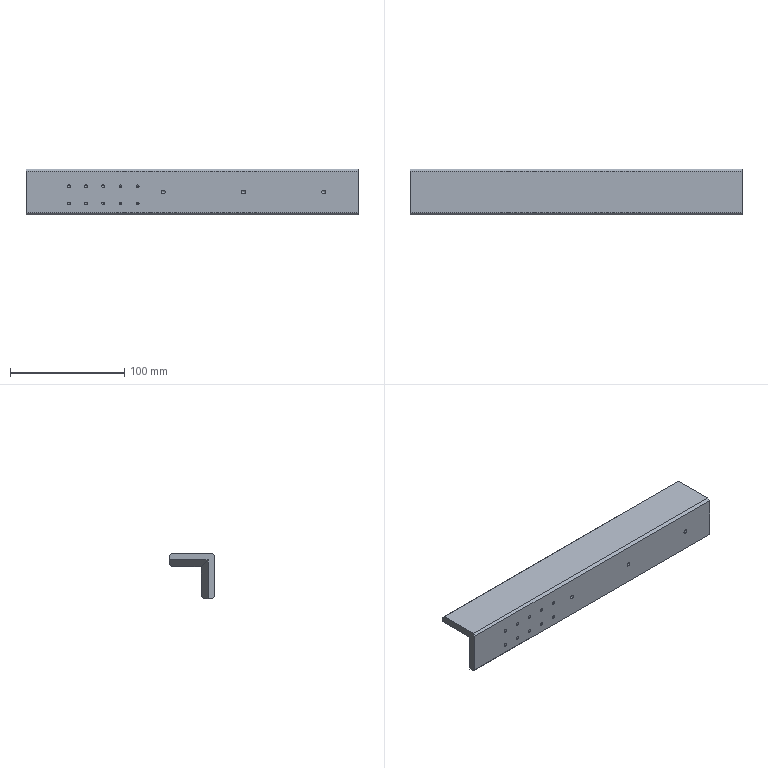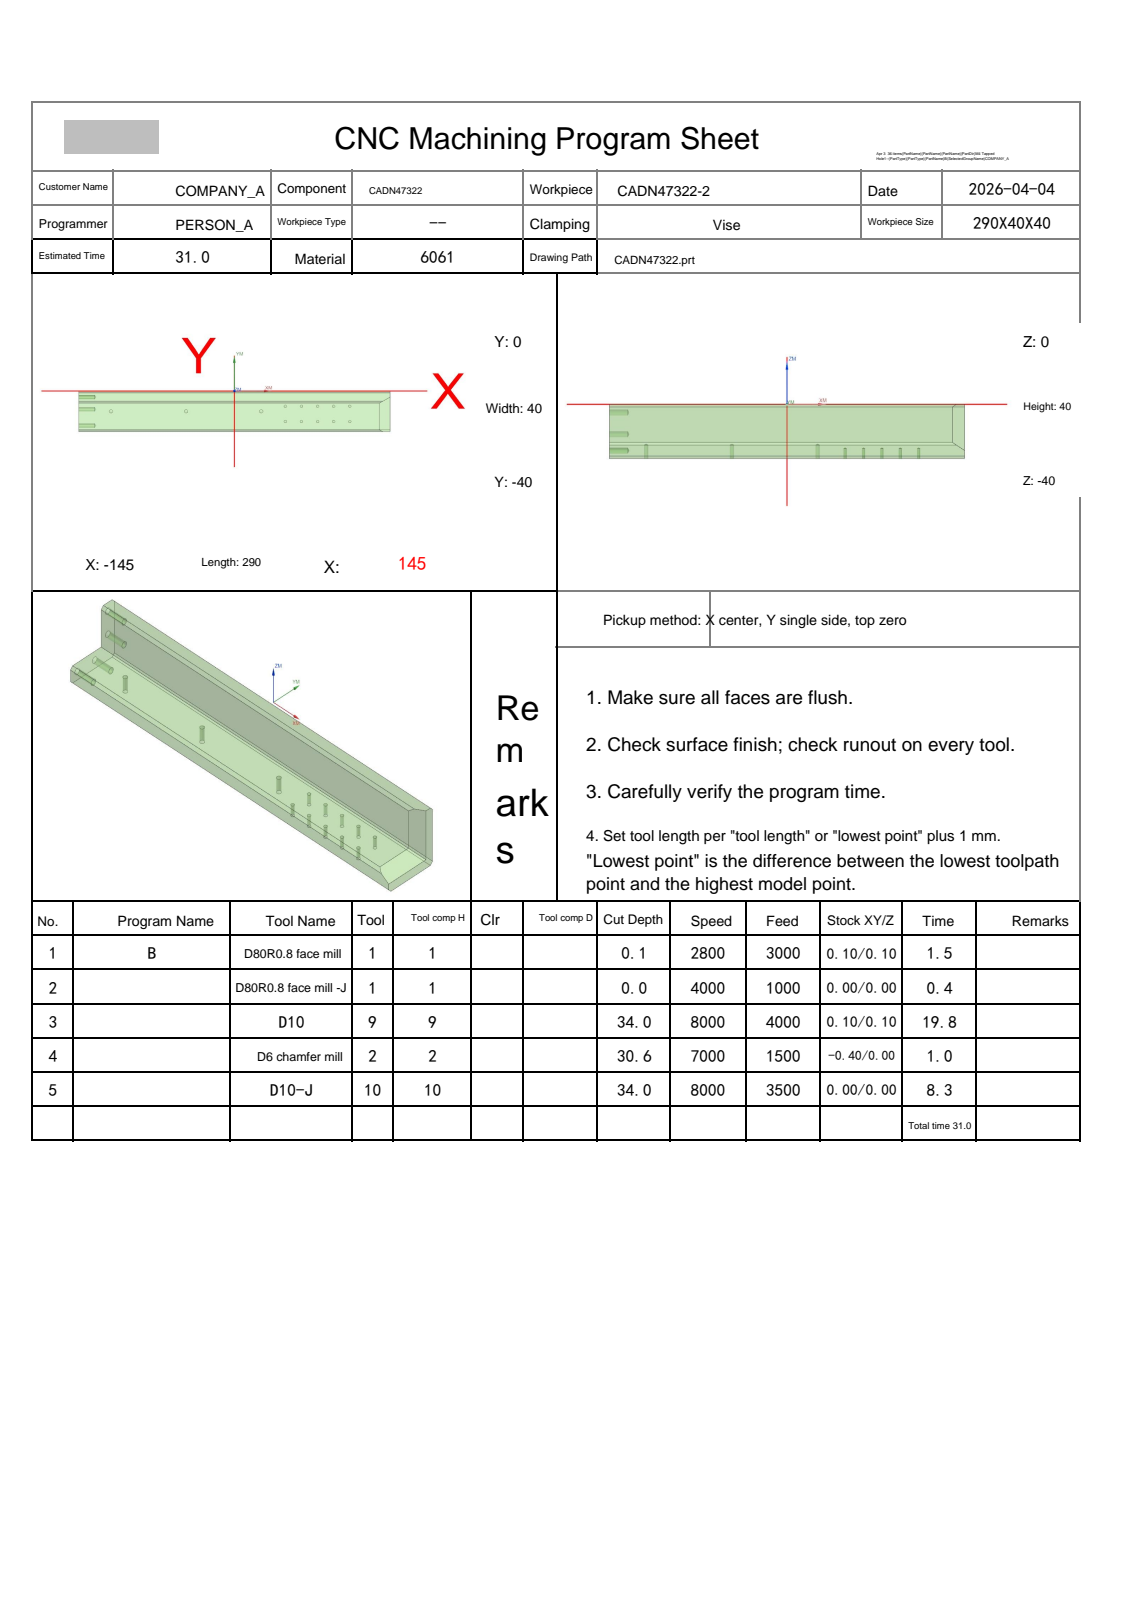NC program | NX | posted by the shop | part box 290 x 40 x 40 mm
Lines 109 to 1290 of 6219:
N3 T09 M06
(D10  D=10. R=0. H=09 ce=0.10 di=0.10)
G00 G90 G54 X8.423 Y-52.151 M03 S8000
G43 H09 Z14.5
M08
Z.503
G01 Z-.698 F4000.
Y-50.
G03 X1.423 Y-43. I-7. J0.0
G01 X-145.08
Y-42.864
Y-17.238
Y-16.914
Y-15.839
X-138.08
X137.115 Y-15.837
G03 X139.795 Y-15.071 I-.184 J5.707
G01 X141.15 Y-14.258
X144.167 Y-12.448
X147.624 Y-10.373
X147.803 Y-10.266
X147.849
X147.905 Y-10.205
X147.981 Y-10.159
G03 X149.252 Y-8.816 I-3.045 J4.154
X150.047 Y-6.732 I-4.252 J2.816
G01 X150.078 Y-6.736
X150.149 Y-6.743
X150.131 Y-6.812
Y-9.995
G02 X148.809 Y-11.288 I-5.195 J3.99
X148.626 Y-11.405 I-.844 J1.121
G01 X148. Y-10.362
Y-10.594
X148.523 Y-11.466
X148.344 Y-11.574
X148. Y-11.78
Y-40.08
X143.456
X143.382 Y-40.73
G02 X142.478 Y-43. I-5.022 J.686
G01 X-.563
G02 X-1.375 Y-42.582 I.001 J1.
G01 X-5.778 Y-36.418
G03 X-6.591 Y-36. I-.813 J-.582
G01 X-137.083
G02 X-138.08 Y-35.004 I.004 J1.
G01 Y-23.835
G02 X-137.084 Y-22.839 I1. J-.004
G01 X137.34 Y-22.834
G03 X139.78 Y-22.517 I-.409 J12.704
G02 X140. Y-22.493 I.22 J-.975
X141. Y-23.489 I0.0 J-1.
G01 Y-32.868
G02 X140.435 Y-33.765 I-1. J.004
G03 X138.046 Y-35.638 I3.021 J-6.314
G02 X137.279 Y-36. I-.77 J.638
G01 X-.913
G02 X-1.619 Y-35.708 I.001 J1.
G01 X-5.534 Y-31.793
G03 X-6.241 Y-31.5 I-.707 J-.707
G01 X-132.584
G02 X-133.58 Y-30.504 I.004 J1.
G01 Y-28.335
G02 X-132.584 Y-27.339 I1. J-.004
G01 X135.504 Y-27.334
G02 X136.5 Y-28.329 I-.004 J-1.
G01 Y-30.443
G02 X136.14 Y-31.207 I-1. J.004
G01 X136.065 Y-31.269
G02 X135.43 Y-31.5 I-.639 J.769
G01 X-3.577
X-4.077
G03 X-11.077 Y-38.5 I0.0 J-7.
G01 Y-52.151
Z.503
G00 Z3.
G01 X8.423 F6000.
G00 Z-.195
G01 Z-1.395 F4000.
Y-50.
G03 X1.423 Y-43. I-7. J0.0
G01 X-145.08
Y-42.864
Y-17.102
Y-16.914
Y-16.535
X-138.08 Y-16.536
X135.891
G03 X138.632 Y-15.768 I-.172 J5.89
G01 X147.625 Y-10.372
X147.803 Y-10.266
X147.849
X147.905 Y-10.205
X147.981 Y-10.159
G03 X149.252 Y-8.816 I-3.045 J4.154
X150.047 Y-6.732 I-4.252 J2.816
G01 X150.078 Y-6.736
X150.149 Y-6.743
X150.131 Y-6.812
Y-9.995
G02 X148.809 Y-11.288 I-5.195 J3.99
X148.626 Y-11.405 I-.844 J1.121
G01 X148. Y-10.362
Y-10.594
X148.523 Y-11.466
X148.344 Y-11.574
X148. Y-11.78
Y-40.08
X143.456
X143.382 Y-40.73
G02 X142.478 Y-43. I-5.022 J.686
G01 X-3.577
G02 X-4.548 Y-42.238 I0.0 J1.
G01 X-5.89 Y-36.761
G03 X-6.861 Y-36. I-.971 J-.239
G01 X-137.084
G02 X-138.08 Y-35.004 I.004 J1.
G01 Y-24.532
G02 X-137.084 Y-23.536 I1. J-.004
G01 X136.095 Y-23.533
G03 X139.695 Y-22.91 I-.376 J12.887
G02 X140. Y-22.863 I.305 J-.952
X141. Y-23.859 I0.0 J-1.
G01 Y-32.869
G02 X140.435 Y-33.765 I-1. J.004
G03 X138.046 Y-35.638 I3.021 J-6.315
G02 X137.28 Y-36. I-.77 J.638
G01 X-.913
G02 X-1.619 Y-35.708 I.001 J1.
G01 X-5.534 Y-31.793
G03 X-6.241 Y-31.5 I-.707 J-.707
G01 X-132.585
G02 X-133.58 Y-30.505 I.005 J1.
G01 Y-29.032
G02 X-132.585 Y-28.036 I1. J-.005
G01 X135.505 Y-28.033
G02 X136.5 Y-29.029 I-.005 J-1.
G01 Y-30.443
G02 X136.14 Y-31.207 I-1. J.005
G01 X136.065 Y-31.269
G02 X135.431 Y-31.5 I-.639 J.769
G01 X-3.577
X-4.077
G03 X-11.077 Y-38.5 I0.0 J-7.
G01 Y-52.151
Z-.195
G00 Z2.303
G01 X8.423 F6000.
G00 Z-.893
G01 Z-2.093 F4000.
Y-50.
G03 X1.423 Y-43. I-7. J0.0
G01 X-145.08
Y-42.864
Y-17.099
X-138.08 Y-17.1
X135.
G03 X137.624 Y-16.373 I0.0 J5.1
G01 X147.626 Y-10.372
X147.803 Y-10.266
X147.849
X147.905 Y-10.205
X147.981 Y-10.159
G03 X149.252 Y-8.816 I-3.045 J4.154
X150.047 Y-6.732 I-4.252 J2.816
G01 X150.078 Y-6.736
X150.149 Y-6.743
X150.131 Y-6.812
Y-9.995
G02 X148.809 Y-11.288 I-5.195 J3.99
X148.626 Y-11.405 I-.844 J1.121
G01 X148. Y-10.362
Y-10.594
X148.523 Y-11.466
X148.344 Y-11.574
X148. Y-11.78
Y-40.08
X143.456
X143.382 Y-40.73
G02 X142.478 Y-43. I-5.022 J.686
G01 X-3.577
G02 X-4.548 Y-42.238 I0.0 J1.
G01 X-5.89 Y-36.761
G03 X-6.861 Y-36. I-.971 J-.239
G01 X-137.084
G02 X-138.08 Y-35.004 I.004 J1.
G01 Y-25.096
G02 X-137.084 Y-24.1 I1. J-.004
G01 X135.
G03 X139.622 Y-23.182 I0.0 J12.1
G02 X140. Y-23.108 I.378 J-.926
X141. Y-24.104 I0.0 J-1.
G01 Y-32.869
G02 X140.436 Y-33.765 I-1. J.004
G03 X138.046 Y-35.638 I3.021 J-6.315
G02 X137.28 Y-36. I-.77 J.638
G01 X-.913
G02 X-1.619 Y-35.708 I.001 J1.
G01 X-5.534 Y-31.793
G03 X-6.241 Y-31.5 I-.707 J-.707
G01 X-132.585
G02 X-133.58 Y-30.505 I.005 J1.
G01 Y-29.595
G02 X-132.585 Y-28.6 I1. J-.005
G01 X135.
G03 X135.476 Y-28.593 I0.0 J16.6
G01 X135.5
G02 X136.5 Y-29.588 I0.0 J-1.
G01 Y-30.443
G02 X136.14 Y-31.207 I-1. J.005
G01 X136.065 Y-31.269
G02 X135.431 Y-31.5 I-.639 J.769
G01 X-3.577
X-4.077
G03 X-11.077 Y-38.5 I0.0 J-7.
G01 Y-52.151
Z-.893
G00 Z1.605
G01 X8.423 F6000.
G00 Z-1.59
G01 Z-2.79 F4000.
Y-50.
G03 X1.423 Y-43. I-7. J0.0
G01 X-145.08
Y-42.864
Y-18.5
Y-17.099
X-138.08 Y-17.1
X135.
G03 X137.624 Y-16.373 I0.0 J5.1
G01 X147.626 Y-10.372
X147.803 Y-10.266
X147.849
X147.905 Y-10.205
X147.981 Y-10.159
G03 X149.252 Y-8.816 I-3.045 J4.154
X150.047 Y-6.732 I-4.252 J2.816
G01 X150.078 Y-6.736
X150.149 Y-6.743
X150.131 Y-6.812
Y-9.995
G02 X148.809 Y-11.288 I-5.195 J3.99
X148.626 Y-11.405 I-.844 J1.121
G01 X148. Y-10.362
Y-10.594
X148.523 Y-11.466
X148.344 Y-11.574
X148. Y-11.78
Y-40.08
X143.456
X143.382 Y-40.73
G02 X142.478 Y-43. I-5.022 J.686
G01 X-3.577
G02 X-4.548 Y-42.238 I0.0 J1.
G01 X-5.89 Y-36.761
G03 X-6.861 Y-36. I-.971 J-.239
G01 X-137.084
G02 X-138.08 Y-35.005 I.005 J1.
G01 Y-25.095
G02 X-137.085 Y-24.1 I1. J-.005
G01 X135.
G03 X139.622 Y-23.182 I0.0 J12.1
G02 X140. Y-23.108 I.378 J-.926
X141. Y-24.104 I0.0 J-1.
G01 Y-32.869
G02 X140.436 Y-33.765 I-1. J.005
G03 X138.046 Y-35.638 I3.02 J-6.315
G02 X137.28 Y-36. I-.77 J.638
G01 X-.913
G02 X-1.619 Y-35.708 I.001 J1.
G01 X-5.534 Y-31.793
G03 X-6.241 Y-31.5 I-.707 J-.707
G01 X-132.585
G02 X-133.58 Y-30.505 I.005 J1.
G01 Y-29.595
G02 X-132.585 Y-28.6 I1. J-.005
G01 X135.
G03 X135.477 Y-28.593 I0.0 J16.6
G01 X135.5
G02 X136.5 Y-29.588 I0.0 J-1.
G01 Y-30.444
G02 X136.14 Y-31.207 I-1. J.005
G01 X136.065 Y-31.27
G02 X135.431 Y-31.5 I-.639 J.77
G01 X-3.577
X-4.077
G03 X-11.077 Y-38.5 I0.0 J-7.
G01 Y-52.151
Z-1.59
G00 Z.908
G01 X8.423 F6000.
G00 Z-2.288
G01 Z-3.488 F4000.
Y-50.
G03 X1.423 Y-43. I-7. J0.0
G01 X-145.08
Y-42.864
Y-17.099
X-138.08 Y-17.1
X135.
G03 X137.624 Y-16.373 I0.0 J5.1
G01 X147.626 Y-10.372
X147.803 Y-10.266
X147.849
X147.905 Y-10.205
X147.981 Y-10.159
G03 X149.252 Y-8.816 I-3.045 J4.154
X150.047 Y-6.732 I-4.252 J2.816
G01 X150.078 Y-6.736
X150.149 Y-6.743
X150.131 Y-6.812
Y-9.995
G02 X148.809 Y-11.288 I-5.195 J3.99
X148.626 Y-11.405 I-.844 J1.121
G01 X148. Y-10.362
Y-10.594
X148.523 Y-11.466
X148.344 Y-11.574
X148. Y-11.78
Y-40.08
X143.456
X143.382 Y-40.73
G02 X142.478 Y-43. I-5.022 J.686
G01 X-3.577
G02 X-4.548 Y-42.238 I0.0 J1.
G01 X-5.89 Y-36.761
G03 X-6.861 Y-36. I-.971 J-.239
G01 X-137.085
G02 X-138.08 Y-35.005 I.005 J1.
G01 Y-25.095
G02 X-137.085 Y-24.1 I1. J-.005
G01 X135.
G03 X139.623 Y-23.182 I0.0 J12.1
G02 X140. Y-23.108 I.377 J-.926
X141. Y-24.103 I0.0 J-1.
G01 Y-32.87
G02 X140.436 Y-33.765 I-1. J.005
G03 X138.045 Y-35.638 I3.02 J-6.315
G02 X137.281 Y-36. I-.77 J.638
G01 X-.913
G02 X-1.619 Y-35.708 I.001 J1.
G01 X-5.534 Y-31.793
G03 X-6.241 Y-31.5 I-.707 J-.707
G01 X-132.585
G02 X-133.58 Y-30.505 I.005 J1.
G01 Y-29.595
G02 X-132.585 Y-28.6 I1. J-.005
G01 X135.
G03 X135.477 Y-28.593 I0.0 J16.6
G01 X135.5
G02 X136.5 Y-29.587 I0.0 J-1.
G01 Y-30.444
G02 X136.14 Y-31.207 I-1. J.005
G01 X136.065 Y-31.27
G02 X135.432 Y-31.5 I-.638 J.77
G01 X-3.577
X-4.077
G03 X-11.077 Y-38.5 I0.0 J-7.
G01 Y-52.151
Z-2.288
G00 Z.21
G01 X8.423 F6000.
G00 Z-2.985
G01 Z-4.185 F4000.
Y-50.
G03 X1.423 Y-43. I-7. J0.0
G01 X-145.08
Y-42.864
Y-18.5
Y-17.099
X-138.08 Y-17.1
X135.
G03 X137.624 Y-16.373 I0.0 J5.1
G01 X147.803 Y-10.266
X147.849
X147.905 Y-10.205
X147.981 Y-10.159
G03 X149.252 Y-8.816 I-3.045 J4.154
X150.047 Y-6.732 I-4.252 J2.816
G01 X150.078 Y-6.736
X150.149 Y-6.743
X150.131 Y-6.812
Y-9.995
G02 X148.809 Y-11.288 I-5.195 J3.99
X148.626 Y-11.405 I-.844 J1.121
G01 X148. Y-10.362
Y-10.594
X148.523 Y-11.466
X148.344 Y-11.574
X148. Y-11.78
Y-40.08
X143.456
X143.382 Y-40.73
G02 X142.478 Y-43. I-5.022 J.686
G01 X-3.577
G02 X-4.548 Y-42.238 I0.0 J1.
G01 X-5.89 Y-36.761
G03 X-6.861 Y-36. I-.971 J-.239
G01 X-137.085
G02 X-138.08 Y-35.005 I.005 J1.
G01 Y-25.095
G02 X-137.085 Y-24.1 I1. J-.005
G01 X135.
G03 X139.623 Y-23.182 I0.0 J12.1
G02 X140. Y-23.108 I.377 J-.926
X141. Y-24.103 I0.0 J-1.
G01 Y-32.87
G02 X140.436 Y-33.764 I-1. J.005
G03 X138.045 Y-35.639 I3.02 J-6.315
G02 X137.281 Y-36. I-.769 J.639
G01 X-.913
G02 X-1.619 Y-35.708 I.001 J1.
G01 X-5.534 Y-31.793
G03 X-6.241 Y-31.5 I-.707 J-.707
G01 X-132.586
G02 X-133.58 Y-30.506 I.006 J1.
G01 Y-29.594
G02 X-132.586 Y-28.6 I1. J-.006
G01 X135.
G03 X135.477 Y-28.593 I0.0 J16.6
G01 X135.5
G02 X136.5 Y-29.587 I0.0 J-1.
G01 Y-30.444
G02 X136.141 Y-31.206 I-1. J.006
G01 X136.064 Y-31.27
G02 X135.432 Y-31.5 I-.638 J.77
G01 X-3.577
X-4.077
G03 X-11.077 Y-38.5 I0.0 J-7.
G01 Y-52.151
Z-2.985
G00 Z-.488
G01 X8.423 F6000.
G00 Z-3.683
G01 Z-4.883 F4000.
Y-50.
G03 X1.423 Y-43. I-7. J0.0
G01 X-145.08
Y-42.864
Y-17.099
X-138.08 Y-17.1
X135.
G03 X137.624 Y-16.373 I0.0 J5.1
G01 X147.627 Y-10.372
X147.803 Y-10.266
X147.849
X147.905 Y-10.205
X147.981 Y-10.159
G03 X149.252 Y-8.816 I-3.045 J4.154
X150.047 Y-6.732 I-4.252 J2.816
G01 X150.078 Y-6.736
X150.149 Y-6.743
X150.131 Y-6.812
Y-9.995
G02 X148.809 Y-11.288 I-5.195 J3.99
X148.626 Y-11.405 I-.844 J1.121
G01 X148. Y-10.362
Y-10.594
X148.523 Y-11.466
X148.344 Y-11.574
X148. Y-11.78
Y-40.08
X143.456
X143.382 Y-40.73
G02 X142.478 Y-43. I-5.022 J.686
G01 X-3.577
G02 X-4.548 Y-42.238 I0.0 J1.
G01 X-5.89 Y-36.761
G03 X-6.861 Y-36. I-.971 J-.239
G01 X-137.085
G02 X-138.08 Y-35.005 I.005 J1.
G01 Y-25.095
G02 X-137.085 Y-24.1 I1. J-.005
G01 X135.
G03 X139.623 Y-23.182 I0.0 J12.1
G02 X140. Y-23.108 I.377 J-.926
X141. Y-24.103 I0.0 J-1.
G01 Y-32.87
G02 X140.437 Y-33.764 I-1. J.005
G03 X138.045 Y-35.639 I3.02 J-6.315
G02 X137.281 Y-36. I-.769 J.639
G01 X-.913
G02 X-1.619 Y-35.708 I.001 J1.
G01 X-5.534 Y-31.793
G03 X-6.241 Y-31.5 I-.707 J-.707
G01 X-132.586
G02 X-133.58 Y-30.506 I.006 J1.
G01 Y-29.594
G02 X-132.586 Y-28.6 I1. J-.006
G01 X135.
G03 X135.477 Y-28.593 I0.0 J16.6
G01 X135.5
G02 X136.5 Y-29.587 I0.0 J-1.
G01 Y-30.445
G02 X136.141 Y-31.206 I-1. J.006
G01 X136.064 Y-31.27
G02 X135.432 Y-31.5 I-.638 J.77
G01 X-3.577
X-4.077
G03 X-11.077 Y-38.5 I0.0 J-7.
G01 Y-52.151
Z-3.683
G00 Z-1.185
G01 X8.423 F6000.
G00 Z-4.38
G01 Z-5.58 F4000.
Y-50.
G03 X1.423 Y-43. I-7. J0.0
G01 X-145.08
Y-42.864
Y-17.099
X-138.08 Y-17.1
X135.
G03 X137.624 Y-16.373 I0.0 J5.1
G01 X147.627 Y-10.371
X147.803 Y-10.266
X147.849
X147.905 Y-10.205
X147.981 Y-10.159
G03 X149.252 Y-8.816 I-3.045 J4.154
X150.047 Y-6.732 I-4.252 J2.816
G01 X150.078 Y-6.736
X150.149 Y-6.743
X150.131 Y-6.812
Y-9.995
G02 X148.809 Y-11.288 I-5.195 J3.99
X148.626 Y-11.405 I-.844 J1.121
G01 X148. Y-10.362
Y-10.594
X148.523 Y-11.466
X148.344 Y-11.574
X148. Y-11.78
Y-40.08
X143.456
X143.382 Y-40.73
G02 X142.478 Y-43. I-5.022 J.686
G01 X-3.577
G02 X-4.548 Y-42.238 I0.0 J1.
G01 X-5.89 Y-36.761
G03 X-6.861 Y-36. I-.971 J-.239
G01 X-137.086
G02 X-138.08 Y-35.006 I.006 J1.
G01 Y-25.094
G02 X-137.086 Y-24.1 I1. J-.006
G01 X135.
G03 X139.623 Y-23.182 I0.0 J12.1
G02 X140. Y-23.108 I.377 J-.926
X141. Y-24.103 I0.0 J-1.
G01 Y-32.87
G02 X140.437 Y-33.764 I-1. J.006
G03 X138.045 Y-35.639 I3.019 J-6.315
G02 X137.281 Y-36. I-.769 J.639
G01 X-.913
G02 X-1.619 Y-35.708 I.001 J1.
G01 X-5.534 Y-31.793
G03 X-6.241 Y-31.5 I-.707 J-.707
G01 X-132.586
G02 X-133.58 Y-30.506 I.006 J1.
G01 Y-29.594
G02 X-132.586 Y-28.6 I1. J-.006
G01 X135.
G03 X135.478 Y-28.593 I0.0 J16.6
G01 X135.5
G02 X136.5 Y-29.587 I0.0 J-1.
G01 Y-30.445
G02 X136.141 Y-31.206 I-1. J.006
G01 X136.064 Y-31.27
G02 X135.432 Y-31.5 I-.638 J.77
G01 X-3.577
X-4.077
G03 X-11.077 Y-38.5 I0.0 J-7.
G01 Y-52.151
Z-4.38
G00 Z-1.883
G01 X8.423 F6000.
G00 Z-5.078
G01 Z-6.278 F4000.
Y-50.
G03 X1.423 Y-43. I-7. J0.0
G01 X-145.08
Y-42.864
Y-17.099
X-138.08 Y-17.1
X135.
G03 X137.624 Y-16.373 I0.0 J5.1
G01 X147.803 Y-10.266
X147.849
X147.905 Y-10.205
X147.981 Y-10.159
G03 X149.252 Y-8.816 I-3.045 J4.154
X150.047 Y-6.732 I-4.252 J2.816
G01 X150.078 Y-6.736
X150.149 Y-6.743
X150.131 Y-6.812
Y-9.995
G02 X148.809 Y-11.288 I-5.195 J3.99
X148.626 Y-11.405 I-.844 J1.121
G01 X148. Y-10.362
Y-10.594
X148.523 Y-11.466
X148.344 Y-11.574
X148. Y-11.78
Y-40.08
X143.456
X143.382 Y-40.73
G02 X142.478 Y-43. I-5.022 J.686
G01 X-3.577
G02 X-4.548 Y-42.238 I0.0 J1.
G01 X-5.89 Y-36.761
G03 X-6.861 Y-36. I-.971 J-.239
G01 X-137.086
G02 X-138.08 Y-35.006 I.006 J1.
G01 Y-25.094
G02 X-137.086 Y-24.1 I1. J-.006
G01 X135.
G03 X139.624 Y-23.182 I0.0 J12.1
G02 X140. Y-23.108 I.376 J-.926
X141. Y-24.102 I0.0 J-1.
G01 Y-32.871
G02 X140.437 Y-33.764 I-1. J.006
G03 X138.045 Y-35.639 I3.019 J-6.315
G02 X137.282 Y-36. I-.769 J.639
G01 X-.913
G02 X-1.619 Y-35.708 I.001 J1.
G01 X-5.534 Y-31.793
G03 X-6.241 Y-31.5 I-.707 J-.707
G01 X-132.586
G02 X-133.58 Y-30.506 I.006 J1.
G01 Y-29.594
G02 X-132.586 Y-28.6 I1. J-.006
G01 X135.
G03 X135.478 Y-28.593 I0.0 J16.6
G01 X135.5
G02 X136.5 Y-29.586 I0.0 J-1.
G01 Y-30.445
G02 X136.141 Y-31.206 I-1. J.006
G01 X136.064 Y-31.27
G02 X135.433 Y-31.5 I-.638 J.77
G01 X-3.577
X-4.077
G03 X-11.077 Y-38.5 I0.0 J-7.
G01 Y-52.151
Z-5.078
G00 Z-2.58
G01 X8.423 F6000.
G00 Z-5.775
G01 Z-6.975 F4000.
Y-50.
G03 X1.423 Y-43. I-7. J0.0
G01 X-145.08
Y-42.864
Y-17.099
X-138.08 Y-17.1
X135.
G03 X137.624 Y-16.373 I0.0 J5.1
G01 X141.374 Y-14.123
X147.803 Y-10.266
X147.849
X147.905 Y-10.205
X147.981 Y-10.159
G03 X149.252 Y-8.816 I-3.045 J4.154
X150.047 Y-6.732 I-4.252 J2.816
G01 X150.078 Y-6.736
X150.149 Y-6.743
X150.131 Y-6.812
Y-9.995
G02 X148.809 Y-11.288 I-5.195 J3.99
X148.626 Y-11.405 I-.844 J1.121
G01 X148. Y-10.362
Y-10.594
X148.523 Y-11.466
X148.344 Y-11.574
X148. Y-11.78
Y-40.08
X143.456
X143.382 Y-40.73
G02 X142.478 Y-43. I-5.022 J.686
G01 X-3.577
G02 X-4.548 Y-42.238 I0.0 J1.
G01 X-5.89 Y-36.761
G03 X-6.861 Y-36. I-.971 J-.239
G01 X-137.086
G02 X-138.08 Y-35.006 I.006 J1.
G01 Y-25.094
G02 X-137.086 Y-24.1 I1. J-.006
G01 X135.
G03 X139.624 Y-23.182 I0.0 J12.1
G02 X140. Y-23.108 I.376 J-.927
X141. Y-24.102 I0.0 J-1.
G01 Y-32.871
G02 X140.437 Y-33.764 I-1. J.006
G03 X138.045 Y-35.639 I3.019 J-6.315
G02 X137.282 Y-36. I-.769 J.639
G01 X-.914
G02 X-1.619 Y-35.708 I.001 J1.
G01 X-5.534 Y-31.793
G03 X-6.241 Y-31.5 I-.707 J-.707
G01 X-132.587
G02 X-133.58 Y-30.507 I.007 J1.
G01 Y-29.593
G02 X-132.587 Y-28.6 I1. J-.007
G01 X135.
G03 X135.478 Y-28.593 I0.0 J16.6
G01 X135.5
G02 X136.5 Y-29.586 I0.0 J-1.
G01 Y-30.445
G02 X136.141 Y-31.206 I-1. J.007
G01 X136.064 Y-31.27
G02 X135.433 Y-31.5 I-.638 J.77
G01 X-3.577
X-4.077
G03 X-11.077 Y-38.5 I0.0 J-7.
G01 Y-52.151
Z-5.775
G00 Z-3.278
G01 X8.423 F6000.
G00 Z-6.473
G01 Z-7.673 F4000.
Y-50.
G03 X1.423 Y-43. I-7. J0.0
G01 X-145.08
Y-42.864
Y-18.5
Y-17.099
X-138.08 Y-17.1
X135.
G03 X137.624 Y-16.373 I0.0 J5.1
G01 X147.628 Y-10.371
X147.803 Y-10.266
X147.849
X147.905 Y-10.205
X147.981 Y-10.159
G03 X149.252 Y-8.816 I-3.045 J4.154
X150.047 Y-6.732 I-4.252 J2.816
G01 X150.078 Y-6.736
X150.149 Y-6.743
X150.131 Y-6.812
Y-9.995
G02 X148.809 Y-11.288 I-5.195 J3.99
X148.626 Y-11.405 I-.844 J1.121
G01 X148. Y-10.362
Y-10.594
X148.523 Y-11.466
X148.344 Y-11.574
X148. Y-11.78
Y-40.08
X143.456
X143.382 Y-40.73
G02 X142.478 Y-43. I-5.022 J.686
G01 X-3.577
G02 X-4.548 Y-42.238 I0.0 J1.
G01 X-5.89 Y-36.761
G03 X-6.861 Y-36. I-.971 J-.239
G01 X-137.086
G02 X-138.08 Y-35.006 I.006 J1.
G01 Y-25.094
G02 X-137.086 Y-24.1 I1. J-.006
G01 X135.
G03 X139.624 Y-23.182 I0.0 J12.1
G02 X140. Y-23.108 I.376 J-.927
X141. Y-24.102 I0.0 J-1.
G01 Y-32.871
G02 X140.437 Y-33.764 I-1. J.006
G03 X138.045 Y-35.64 I3.019 J-6.316
G02 X137.282 Y-36. I-.769 J.64
G01 X-.913
G02 X-1.619 Y-35.708 I.001 J1.
G01 X-5.534 Y-31.793
G03 X-6.241 Y-31.5 I-.707 J-.707
G01 X-132.587
G02 X-133.58 Y-30.507 I.007 J1.
G01 Y-29.593
G02 X-132.587 Y-28.6 I1. J-.007
G01 X135.
G03 X135.478 Y-28.593 I0.0 J16.6
G01 X135.5
G02 X136.5 Y-29.586 I0.0 J-1.
G01 Y-30.445
G02 X136.142 Y-31.206 I-1. J.007
G01 X136.064 Y-31.271
G02 X135.433 Y-31.5 I-.637 J.771
G01 X-3.577
X-4.077
G03 X-11.077 Y-38.5 I0.0 J-7.
G01 Y-52.151
Z-6.473
G00 Z-3.975
G01 X8.423 F6000.
G00 Z-7.17
G01 Z-8.37 F4000.
Y-50.
G03 X1.423 Y-43. I-7. J0.0
G01 X-145.08
Y-42.864
Y-17.099
X-138.08 Y-17.1
X135.
G03 X137.624 Y-16.373 I0.0 J5.1
G01 X147.628 Y-10.371
X147.803 Y-10.266
X147.849
X147.905 Y-10.205
X147.981 Y-10.159
G03 X149.252 Y-8.816 I-3.045 J4.154
X150.047 Y-6.732 I-4.252 J2.816
G01 X150.078 Y-6.736
X150.149 Y-6.743
X150.131 Y-6.812
Y-9.995
G02 X148.809 Y-11.288 I-5.195 J3.99
X148.626 Y-11.405 I-.844 J1.121
G01 X148. Y-10.362
Y-10.594
X148.523 Y-11.466
X148.344 Y-11.574
X148. Y-11.78
Y-40.08
X143.456
X143.382 Y-40.73
G02 X142.478 Y-43. I-5.022 J.686
G01 X-3.577
G02 X-4.548 Y-42.238 I0.0 J1.
G01 X-5.89 Y-36.761
G03 X-6.861 Y-36. I-.971 J-.239
G01 X-137.087
G02 X-138.08 Y-35.007 I.007 J1.
G01 Y-25.093
G02 X-137.087 Y-24.1 I1. J-.007
G01 X135.
G03 X139.624 Y-23.182 I0.0 J12.1
G02 X140. Y-23.108 I.376 J-.927
X141. Y-24.102 I0.0 J-1.
G01 Y-32.871
G02 X140.438 Y-33.764 I-1. J.007
G03 X138.044 Y-35.64 I3.019 J-6.316
G02 X137.282 Y-36. I-.769 J.64
G01 X-.913
G02 X-1.619 Y-35.708 I.001 J1.
G01 X-5.534 Y-31.793
G03 X-6.241 Y-31.5 I-.707 J-.707
G01 X-132.587
G02 X-133.58 Y-30.507 I.007 J1.
G01 Y-29.593
G02 X-132.587 Y-28.6 I1. J-.007
G01 X135.
G03 X135.478 Y-28.593 I0.0 J16.6
G01 X135.5
G02 X136.5 Y-29.586 I0.0 J-1.
G01 Y-30.446
G02 X136.142 Y-31.206 I-1. J.007
G01 X136.063 Y-31.271
G02 X135.433 Y-31.5 I-.637 J.771
G01 X-3.577
X-4.077
G03 X-11.077 Y-38.5 I0.0 J-7.
G01 Y-52.151
Z-7.17
G00 Z-4.673
G01 X8.423 F6000.
G00 Z-7.868
G01 Z-9.068 F4000.
Y-50.
G03 X1.423 Y-43. I-7. J0.0
G01 X-145.08
Y-42.864
Y-18.5
Y-17.099
X-138.08 Y-17.1
X135.
G03 X137.624 Y-16.373 I0.0 J5.1
G01 X147.628 Y-10.371
X147.803 Y-10.266
X147.849
X147.905 Y-10.205
X147.981 Y-10.159
G03 X149.252 Y-8.816 I-3.045 J4.154
X150.047 Y-6.732 I-4.252 J2.816
G01 X150.078 Y-6.736
X150.149 Y-6.743
X150.131 Y-6.812
Y-9.995
G02 X148.809 Y-11.288 I-5.195 J3.99
X148.626 Y-11.405 I-.844 J1.121
G01 X148. Y-10.362
Y-10.594
X148.523 Y-11.466
X148.344 Y-11.574
X148. Y-11.78
Y-40.08
X143.456
X143.382 Y-40.73
G02 X142.478 Y-43. I-5.022 J.686
G01 X-3.577
G02 X-4.548 Y-42.238 I0.0 J1.
G01 X-5.89 Y-36.761
G03 X-6.861 Y-36. I-.971 J-.239
G01 X-137.087
G02 X-138.08 Y-35.007 I.007 J1.
G01 Y-25.093
G02 X-137.087 Y-24.1 I1. J-.007
G01 X135.
G03 X139.624 Y-23.181 I0.0 J12.1
G02 X140. Y-23.108 I.376 J-.927
X141. Y-24.101 I0.0 J-1.
G01 Y-32.872
G02 X140.438 Y-33.764 I-1. J.007
G03 X138.044 Y-35.64 I3.018 J-6.316
G02 X137.283 Y-36. I-.768 J.64
G01 X-.913
G02 X-1.619 Y-35.708 I.001 J1.
G01 X-5.534 Y-31.793
G03 X-6.241 Y-31.5 I-.707 J-.707
G01 X-132.587
G02 X-133.58 Y-30.507 I.007 J1.
G01 Y-29.593
G02 X-132.587 Y-28.6 I1. J-.007
G01 X135.
G03 X135.479 Y-28.593 I0.0 J16.6
G01 X135.5
G02 X136.5 Y-29.586 I0.0 J-1.
G01 Y-30.446
G02 X136.142 Y-31.205 I-1. J.007
G01 X136.063 Y-31.271
G02 X135.433 Y-31.5 I-.637 J.771
G01 X-3.577
X-4.077
G03 X-11.077 Y-38.5 I0.0 J-7.
G01 Y-52.151
Z-7.868
G00 Z-5.37
G01 X8.423 F6000.
G00 Z-8.565
G01 Z-9.765 F4000.
Y-50.
G03 X1.423 Y-43. I-7. J0.0
G01 X-145.08
Y-42.864
Y-17.099
X-138.08 Y-17.1
X135.
G03 X137.624 Y-16.373 I0.0 J5.1
G01 X147.803 Y-10.266
X147.849
X147.905 Y-10.205
X147.981 Y-10.159
G03 X149.252 Y-8.816 I-3.045 J4.154
X150.047 Y-6.732 I-4.252 J2.816
G01 X150.078 Y-6.736
X150.149 Y-6.743
X150.131 Y-6.812
Y-9.995
G02 X148.809 Y-11.288 I-5.195 J3.99
X148.626 Y-11.405 I-.844 J1.121
G01 X148. Y-10.362
Y-10.594
X148.523 Y-11.466
X148.344 Y-11.574
X148. Y-11.78
Y-40.08
X143.456
X143.382 Y-40.73
G02 X142.478 Y-43. I-5.022 J.686
G01 X-3.577
G02 X-4.548 Y-42.238 I0.0 J1.
G01 X-5.89 Y-36.761
G03 X-6.861 Y-36. I-.971 J-.239
G01 X-137.087
G02 X-138.08 Y-35.007 I.007 J1.
G01 Y-25.093
G02 X-137.087 Y-24.1 I1. J-.007
G01 X135.
G03 X139.625 Y-23.181 I0.0 J12.1
G02 X140. Y-23.108 I.375 J-.927
X141. Y-24.101 I0.0 J-1.
G01 Y-32.872
G02 X140.438 Y-33.764 I-1. J.007
G03 X138.044 Y-35.64 I3.018 J-6.316
G02 X137.283 Y-36. I-.768 J.64
G01 X-.913
G02 X-1.619 Y-35.708 I.001 J1.
G01 X-5.534 Y-31.793
G03 X-6.241 Y-31.5 I-.707 J-.707
G01 X-132.587
G02 X-133.58 Y-30.507 I.007 J1.
G01 Y-29.593
G02 X-132.587 Y-28.6 I1. J-.007
G01 X135.
G03 X135.479 Y-28.593 I0.0 J16.6
G01 X135.5
G02 X136.5 Y-29.585 I0.0 J-1.
G01 Y-30.446
G02 X136.142 Y-31.205 I-1. J.007
G01 X136.063 Y-31.271
G02 X135.434 Y-31.5 I-.637 J.771
G01 X-3.577
X-4.077
G03 X-11.077 Y-38.5 I0.0 J-7.
G01 Y-52.151
Z-8.565
G00 Z-6.068
G01 X8.423 F6000.
G00 Z-9.263
G01 Z-10.463 F4000.
Y-50.
G03 X1.423 Y-43. I-7. J0.0
G01 X-145.08
Y-42.864
Y-17.099
X-138.08 Y-17.1
X135.
G03 X137.624 Y-16.373 I0.0 J5.1
G01 X147.628 Y-10.371
X147.803 Y-10.266
X147.849
X147.905 Y-10.205
X147.981 Y-10.159
G03 X149.252 Y-8.816 I-3.045 J4.154
X150.047 Y-6.732 I-4.252 J2.816
G01 X150.078 Y-6.736
X150.149 Y-6.743
X150.131 Y-6.812
Y-9.995
G02 X148.809 Y-11.288 I-5.195 J3.99
X148.626 Y-11.405 I-.844 J1.121
G01 X148. Y-10.362
Y-10.594
X148.523 Y-11.466
X148.344 Y-11.574
X148. Y-11.78
Y-40.08
X143.456
X143.382 Y-40.73
G02 X142.478 Y-43. I-5.022 J.686
G01 X-3.577
G02 X-4.548 Y-42.238 I0.0 J1.
G01 X-5.89 Y-36.761
G03 X-6.861 Y-36. I-.971 J-.239
G01 X-137.087
G02 X-138.08 Y-35.007 I.007 J1.
G01 Y-25.093
G02 X-137.087 Y-24.1 I1. J-.007
G01 X135.
G03 X139.625 Y-23.181 I0.0 J12.1
G02 X140. Y-23.108 I.375 J-.927
X141. Y-24.101 I0.0 J-1.
G01 Y-32.872
G02 X140.438 Y-33.764 I-1. J.007
G03 X138.044 Y-35.64 I3.018 J-6.316
G02 X137.283 Y-36. I-.768 J.64
G01 X-.913
G02 X-1.619 Y-35.708 I.001 J1.
G01 X-5.534 Y-31.793
G03 X-6.241 Y-31.5 I-.707 J-.707
G01 X-132.588
G02 X-133.58 Y-30.508 I.008 J1.
G01 Y-29.592
G02 X-132.588 Y-28.6 I1. J-.008
G01 X135.
G03 X135.479 Y-28.593 I0.0 J16.6
G01 X135.5
G02 X136.5 Y-29.585 I0.0 J-1.
G01 Y-30.446
G02 X136.142 Y-31.205 I-1. J.008
G01 X136.063 Y-31.271
G02 X135.434 Y-31.5 I-.637 J.771
G01 X-3.577
X-4.077
G03 X-11.077 Y-38.5 I0.0 J-7.
G01 Y-52.151
Z-9.263
G00 Z-6.765
G01 X8.423 F6000.
G00 Z-9.96
G01 Z-11.16 F4000.
Y-50.
G03 X1.423 Y-43. I-7. J0.0
G01 X-145.08
Y-42.864
Y-17.099
X-138.08 Y-17.1
X135.
G03 X137.624 Y-16.373 I0.0 J5.1
G01 X147.628 Y-10.371
X147.803 Y-10.266
X147.849
X147.905 Y-10.205
X147.981 Y-10.159
G03 X149.252 Y-8.816 I-3.045 J4.154
X150.047 Y-6.732 I-4.252 J2.816
G01 X150.078 Y-6.736
X150.149 Y-6.743
X150.131 Y-6.812
Y-9.995
G02 X148.809 Y-11.288 I-5.195 J3.99
X148.626 Y-11.405 I-.844 J1.121
G01 X148. Y-10.362
Y-10.594
X148.523 Y-11.466
X148.344 Y-11.574
X148. Y-11.78
Y-40.08
X143.456
X143.382 Y-40.73
G02 X142.478 Y-43. I-5.022 J.686
G01 X-3.577
G02 X-4.548 Y-42.238 I0.0 J1.
G01 X-5.89 Y-36.761
G03 X-6.861 Y-36. I-.971 J-.239
G01 X-137.087
G02 X-138.08 Y-35.007 I.007 J1.
G01 Y-25.093
G02 X-137.087 Y-24.1 I1. J-.007
G01 X135.
G03 X139.625 Y-23.181 I0.0 J12.1
G02 X140. Y-23.108 I.375 J-.927
X141. Y-24.101 I0.0 J-1.
G01 Y-32.872
G02 X140.438 Y-33.764 I-1. J.007
G03 X138.044 Y-35.64 I3.018 J-6.316
G02 X137.283 Y-36. I-.768 J.64
G01 X-.913
G02 X-1.619 Y-35.708 I.001 J1.
G01 X-5.534 Y-31.793
G03 X-6.241 Y-31.5 I-.707 J-.707
G01 X-132.588
G02 X-133.58 Y-30.508 I.008 J1.
G01 Y-29.592
G02 X-132.588 Y-28.6 I1. J-.008
G01 X135.
G03 X135.479 Y-28.593 I0.0 J16.6
G01 X135.5
G02 X136.5 Y-29.585 I0.0 J-1.
G01 Y-30.446
G02 X136.142 Y-31.205 I-1. J.008
G01 X136.063 Y-31.271
G02 X135.434 Y-31.5 I-.637 J.771
G01 X-3.577
X-4.077
G03 X-11.077 Y-38.5 I0.0 J-7.
G01 Y-52.151
Z-9.96
G00 Z-7.463
G01 X8.423 F6000.
G00 Z-10.658
G01 Z-11.858 F4000.
Y-50.
G03 X1.423 Y-43. I-7. J0.0
G01 X-145.08
Y-42.864
Y-18.5
Y-17.099
X-138.08 Y-17.1
X135.
G03 X137.624 Y-16.373 I0.0 J5.1
G01 X147.628 Y-10.37
X147.803 Y-10.266
X147.849
X147.905 Y-10.205
X147.981 Y-10.159
G03 X149.252 Y-8.816 I-3.045 J4.154
X150.047 Y-6.732 I-4.252 J2.816
G01 X150.078 Y-6.736
X150.149 Y-6.743
X150.131 Y-6.812
Y-9.995
G02 X148.809 Y-11.288 I-5.195 J3.99
X148.626 Y-11.405 I-.844 J1.121
G01 X148. Y-10.362
Y-10.594
X148.523 Y-11.466
X148.344 Y-11.574
X148. Y-11.78
Y-40.08
X143.456
X143.382 Y-40.73
G02 X142.478 Y-43. I-5.022 J.686
G01 X-3.577
G02 X-4.548 Y-42.238 I0.0 J1.
G01 X-5.89 Y-36.761
G03 X-6.861 Y-36. I-.971 J-.239
G01 X-137.088